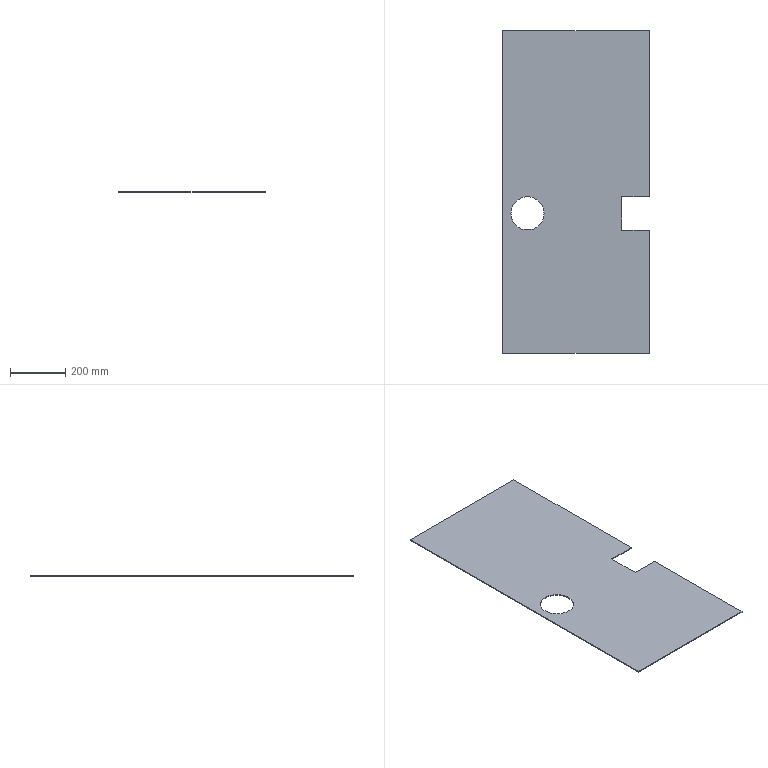Part | SolidWorks | features Cut 1, Extrusion 1 | 1 solid | 12 faces | box 530 x 1165 x 3 mm | volume 1782421 mm3 | plane 10 | cylinder 2 | commonest cylinder face diameters 120 x2
STEP:
#1=CARTESIAN_POINT('',(150.,505.,3.));
#2=VERTEX_POINT('',#1);
#3=CARTESIAN_POINT('',(30.,505.,3.));
#4=VERTEX_POINT('',#3);
#5=CARTESIAN_POINT('',(90.,505.,3.));
#6=DIRECTION('',(0.,0.,-1.));
#7=DIRECTION('',(-1.,0.,0.));
#8=AXIS2_PLACEMENT_3D('',#5,#6,#7);
#9=CIRCLE('',#8,60.);
#10=EDGE_CURVE('',#2,#4,#9,.T.);
#11=ORIENTED_EDGE('',*,*,#10,.F.);
#12=CARTESIAN_POINT('',(150.,505.,0.));
#13=VERTEX_POINT('',#12);
#14=CARTESIAN_POINT('',(150.,505.,10.));
#15=DIRECTION('',(0.,0.,-1.));
#16=VECTOR('',#15,1000.);
#17=LINE('',#14,#16);
#18=EDGE_CURVE('',#2,#13,#17,.T.);
#19=ORIENTED_EDGE('',*,*,#18,.T.);
#20=CARTESIAN_POINT('',(30.,505.,0.));
#21=VERTEX_POINT('',#20);
#22=CARTESIAN_POINT('',(90.,505.,0.));
#23=DIRECTION('',(0.,0.,-1.));
#24=DIRECTION('',(-1.,0.,0.));
#25=AXIS2_PLACEMENT_3D('',#22,#23,#24);
#26=CIRCLE('',#25,60.);
#27=EDGE_CURVE('',#13,#21,#26,.T.);
#28=ORIENTED_EDGE('',*,*,#27,.T.);
#29=CARTESIAN_POINT('',(30.,505.,10.));
#30=DIRECTION('',(0.,0.,-1.));
#31=VECTOR('',#30,1000.);
#32=LINE('',#29,#31);
#33=EDGE_CURVE('',#4,#21,#32,.T.);
#34=ORIENTED_EDGE('',*,*,#33,.F.);
#35=EDGE_LOOP('',(#11,#19,#28,#34));
#36=FACE_OUTER_BOUND('',#35,.T.);
#37=CARTESIAN_POINT('',(90.,505.,10.));
#38=DIRECTION('',(0.,0.,-1.));
#39=DIRECTION('',(-1.,0.,0.));
#40=AXIS2_PLACEMENT_3D('',#37,#38,#39);
#41=CYLINDRICAL_SURFACE('',#40,60.);
#42=ADVANCED_FACE('',(#36),#41,.F.);
#43=CARTESIAN_POINT('',(530.,565.,3.));
#44=VERTEX_POINT('',#43);
#45=CARTESIAN_POINT('',(530.,1165.,3.));
#46=VERTEX_POINT('',#45);
#47=CARTESIAN_POINT('',(530.,0.,3.));
#48=DIRECTION('',(0.,1.,0.));
#49=VECTOR('',#48,1000.);
#50=LINE('',#47,#49);
#51=EDGE_CURVE('',#44,#46,#50,.T.);
#52=ORIENTED_EDGE('',*,*,#51,.F.);
#53=CARTESIAN_POINT('',(530.,565.,0.));
#54=VERTEX_POINT('',#53);
#55=CARTESIAN_POINT('',(530.,565.,3.));
#56=DIRECTION('',(0.,0.,-1.));
#57=VECTOR('',#56,1000.);
#58=LINE('',#55,#57);
#59=EDGE_CURVE('',#44,#54,#58,.T.);
#60=ORIENTED_EDGE('',*,*,#59,.T.);
#61=CARTESIAN_POINT('',(530.,1165.,0.));
#62=VERTEX_POINT('',#61);
#63=CARTESIAN_POINT('',(530.,0.,0.));
#64=DIRECTION('',(0.,1.,0.));
#65=VECTOR('',#64,1000.);
#66=LINE('',#63,#65);
#67=EDGE_CURVE('',#54,#62,#66,.T.);
#68=ORIENTED_EDGE('',*,*,#67,.T.);
#69=CARTESIAN_POINT('',(530.,1165.,3.));
#70=DIRECTION('',(0.,0.,-1.));
#71=VECTOR('',#70,1000.);
#72=LINE('',#69,#71);
#73=EDGE_CURVE('',#46,#62,#72,.T.);
#74=ORIENTED_EDGE('',*,*,#73,.F.);
#75=EDGE_LOOP('',(#52,#60,#68,#74));
#76=FACE_OUTER_BOUND('',#75,.T.);
#77=CARTESIAN_POINT('',(530.,0.,3.));
#78=DIRECTION('',(-1.,0.,0.));
#79=DIRECTION('',(0.,0.,1.));
#80=AXIS2_PLACEMENT_3D('',#77,#78,#79);
#81=PLANE('',#80);
#82=ADVANCED_FACE('',(#76),#81,.F.);
#83=CARTESIAN_POINT('',(0.,1165.,0.));
#84=VERTEX_POINT('',#83);
#85=CARTESIAN_POINT('',(0.,0.,0.));
#86=VERTEX_POINT('',#85);
#87=CARTESIAN_POINT('',(0.,0.,0.));
#88=DIRECTION('',(0.,-1.,0.));
#89=VECTOR('',#88,1000.);
#90=LINE('',#87,#89);
#91=EDGE_CURVE('',#84,#86,#90,.T.);
#92=ORIENTED_EDGE('',*,*,#91,.T.);
#93=CARTESIAN_POINT('',(0.,0.,3.));
#94=VERTEX_POINT('',#93);
#95=CARTESIAN_POINT('',(0.,0.,3.));
#96=DIRECTION('',(0.,0.,-1.));
#97=VECTOR('',#96,1000.);
#98=LINE('',#95,#97);
#99=EDGE_CURVE('',#94,#86,#98,.T.);
#100=ORIENTED_EDGE('',*,*,#99,.F.);
#101=CARTESIAN_POINT('',(0.,1165.,3.));
#102=VERTEX_POINT('',#101);
#103=CARTESIAN_POINT('',(0.,0.,3.));
#104=DIRECTION('',(0.,-1.,0.));
#105=VECTOR('',#104,1000.);
#106=LINE('',#103,#105);
#107=EDGE_CURVE('',#102,#94,#106,.T.);
#108=ORIENTED_EDGE('',*,*,#107,.F.);
#109=CARTESIAN_POINT('',(0.,1165.,3.));
#110=DIRECTION('',(0.,0.,-1.));
#111=VECTOR('',#110,1000.);
#112=LINE('',#109,#111);
#113=EDGE_CURVE('',#102,#84,#112,.T.);
#114=ORIENTED_EDGE('',*,*,#113,.T.);
#115=EDGE_LOOP('',(#92,#100,#108,#114));
#116=FACE_OUTER_BOUND('',#115,.T.);
#117=CARTESIAN_POINT('',(0.,0.,3.));
#118=DIRECTION('',(1.,0.,0.));
#119=DIRECTION('',(0.,0.,-1.));
#120=AXIS2_PLACEMENT_3D('',#117,#118,#119);
#121=PLANE('',#120);
#122=ADVANCED_FACE('',(#116),#121,.F.);
#123=CARTESIAN_POINT('',(530.,0.,0.));
#124=VERTEX_POINT('',#123);
#125=CARTESIAN_POINT('',(0.,0.,0.));
#126=DIRECTION('',(1.,0.,0.));
#127=VECTOR('',#126,1000.);
#128=LINE('',#125,#127);
#129=EDGE_CURVE('',#86,#124,#128,.T.);
#130=ORIENTED_EDGE('',*,*,#129,.T.);
#131=CARTESIAN_POINT('',(530.,0.,3.));
#132=VERTEX_POINT('',#131);
#133=CARTESIAN_POINT('',(530.,0.,3.));
#134=DIRECTION('',(0.,0.,-1.));
#135=VECTOR('',#134,1000.);
#136=LINE('',#133,#135);
#137=EDGE_CURVE('',#132,#124,#136,.T.);
#138=ORIENTED_EDGE('',*,*,#137,.F.);
#139=CARTESIAN_POINT('',(0.,0.,3.));
#140=DIRECTION('',(1.,0.,0.));
#141=VECTOR('',#140,1000.);
#142=LINE('',#139,#141);
#143=EDGE_CURVE('',#94,#132,#142,.T.);
#144=ORIENTED_EDGE('',*,*,#143,.F.);
#145=ORIENTED_EDGE('',*,*,#99,.T.);
#146=EDGE_LOOP('',(#130,#138,#144,#145));
#147=FACE_OUTER_BOUND('',#146,.T.);
#148=CARTESIAN_POINT('',(0.,0.,3.));
#149=DIRECTION('',(0.,1.,0.));
#150=DIRECTION('',(0.,0.,1.));
#151=AXIS2_PLACEMENT_3D('',#148,#149,#150);
#152=PLANE('',#151);
#153=ADVANCED_FACE('',(#147),#152,.F.);
#154=CARTESIAN_POINT('',(530.,445.,0.));
#155=VERTEX_POINT('',#154);
#156=CARTESIAN_POINT('',(530.,0.,0.));
#157=DIRECTION('',(0.,1.,0.));
#158=VECTOR('',#157,1000.);
#159=LINE('',#156,#158);
#160=EDGE_CURVE('',#124,#155,#159,.T.);
#161=ORIENTED_EDGE('',*,*,#160,.T.);
#162=CARTESIAN_POINT('',(530.,445.,3.));
#163=VERTEX_POINT('',#162);
#164=CARTESIAN_POINT('',(530.,445.,3.));
#165=DIRECTION('',(0.,0.,1.));
#166=VECTOR('',#165,1000.);
#167=LINE('',#164,#166);
#168=EDGE_CURVE('',#155,#163,#167,.T.);
#169=ORIENTED_EDGE('',*,*,#168,.T.);
#170=CARTESIAN_POINT('',(530.,0.,3.));
#171=DIRECTION('',(0.,1.,0.));
#172=VECTOR('',#171,1000.);
#173=LINE('',#170,#172);
#174=EDGE_CURVE('',#132,#163,#173,.T.);
#175=ORIENTED_EDGE('',*,*,#174,.F.);
#176=ORIENTED_EDGE('',*,*,#137,.T.);
#177=EDGE_LOOP('',(#161,#169,#175,#176));
#178=FACE_OUTER_BOUND('',#177,.T.);
#179=CARTESIAN_POINT('',(530.,0.,3.));
#180=DIRECTION('',(-1.,0.,0.));
#181=DIRECTION('',(0.,0.,1.));
#182=AXIS2_PLACEMENT_3D('',#179,#180,#181);
#183=PLANE('',#182);
#184=ADVANCED_FACE('',(#178),#183,.F.);
#185=CARTESIAN_POINT('',(0.,1165.,0.));
#186=DIRECTION('',(-1.,0.,0.));
#187=VECTOR('',#186,1000.);
#188=LINE('',#185,#187);
#189=EDGE_CURVE('',#62,#84,#188,.T.);
#190=ORIENTED_EDGE('',*,*,#189,.T.);
#191=ORIENTED_EDGE('',*,*,#113,.F.);
#192=CARTESIAN_POINT('',(0.,1165.,3.));
#193=DIRECTION('',(-1.,0.,0.));
#194=VECTOR('',#193,1000.);
#195=LINE('',#192,#194);
#196=EDGE_CURVE('',#46,#102,#195,.T.);
#197=ORIENTED_EDGE('',*,*,#196,.F.);
#198=ORIENTED_EDGE('',*,*,#73,.T.);
#199=EDGE_LOOP('',(#190,#191,#197,#198));
#200=FACE_OUTER_BOUND('',#199,.T.);
#201=CARTESIAN_POINT('',(0.,1165.,3.));
#202=DIRECTION('',(0.,-1.,0.));
#203=DIRECTION('',(0.,0.,-1.));
#204=AXIS2_PLACEMENT_3D('',#201,#202,#203);
#205=PLANE('',#204);
#206=ADVANCED_FACE('',(#200),#205,.F.);
#207=CARTESIAN_POINT('',(90.,505.,3.));
#208=DIRECTION('',(0.,0.,-1.));
#209=DIRECTION('',(-1.,0.,0.));
#210=AXIS2_PLACEMENT_3D('',#207,#208,#209);
#211=CIRCLE('',#210,60.);
#212=EDGE_CURVE('',#4,#2,#211,.T.);
#213=ORIENTED_EDGE('',*,*,#212,.T.);
#214=ORIENTED_EDGE('',*,*,#10,.T.);
#215=EDGE_LOOP('',(#213,#214));
#216=FACE_BOUND('',#215,.T.);
#217=CARTESIAN_POINT('',(430.,445.,3.));
#218=VERTEX_POINT('',#217);
#219=CARTESIAN_POINT('',(430.,565.,3.));
#220=VERTEX_POINT('',#219);
#221=CARTESIAN_POINT('',(430.,0.,3.));
#222=DIRECTION('',(0.,1.,0.));
#223=VECTOR('',#222,1000.);
#224=LINE('',#221,#223);
#225=EDGE_CURVE('',#218,#220,#224,.T.);
#226=ORIENTED_EDGE('',*,*,#225,.T.);
#227=CARTESIAN_POINT('',(0.,565.,3.));
#228=DIRECTION('',(1.,0.,0.));
#229=VECTOR('',#228,1000.);
#230=LINE('',#227,#229);
#231=EDGE_CURVE('',#220,#44,#230,.T.);
#232=ORIENTED_EDGE('',*,*,#231,.T.);
#233=ORIENTED_EDGE('',*,*,#51,.T.);
#234=ORIENTED_EDGE('',*,*,#196,.T.);
#235=ORIENTED_EDGE('',*,*,#107,.T.);
#236=ORIENTED_EDGE('',*,*,#143,.T.);
#237=ORIENTED_EDGE('',*,*,#174,.T.);
#238=CARTESIAN_POINT('',(0.,445.,3.));
#239=DIRECTION('',(-1.,0.,0.));
#240=VECTOR('',#239,1000.);
#241=LINE('',#238,#240);
#242=EDGE_CURVE('',#163,#218,#241,.T.);
#243=ORIENTED_EDGE('',*,*,#242,.T.);
#244=EDGE_LOOP('',(#226,#232,#233,#234,#235,#236,#237,#243));
#245=FACE_OUTER_BOUND('',#244,.T.);
#246=CARTESIAN_POINT('',(0.,0.,3.));
#247=DIRECTION('',(0.,0.,-1.));
#248=DIRECTION('',(-1.,0.,0.));
#249=AXIS2_PLACEMENT_3D('',#246,#247,#248);
#250=PLANE('',#249);
#251=ADVANCED_FACE('',(#216,#245),#250,.F.);
#252=CARTESIAN_POINT('',(90.,505.,0.));
#253=DIRECTION('',(0.,0.,-1.));
#254=DIRECTION('',(-1.,0.,0.));
#255=AXIS2_PLACEMENT_3D('',#252,#253,#254);
#256=CIRCLE('',#255,60.);
#257=EDGE_CURVE('',#21,#13,#256,.T.);
#258=ORIENTED_EDGE('',*,*,#257,.F.);
#259=ORIENTED_EDGE('',*,*,#27,.F.);
#260=EDGE_LOOP('',(#258,#259));
#261=FACE_BOUND('',#260,.T.);
#262=CARTESIAN_POINT('',(430.,565.,0.));
#263=VERTEX_POINT('',#262);
#264=CARTESIAN_POINT('',(430.,565.,0.));
#265=DIRECTION('',(1.,0.,0.));
#266=VECTOR('',#265,1000.);
#267=LINE('',#264,#266);
#268=EDGE_CURVE('',#263,#54,#267,.T.);
#269=ORIENTED_EDGE('',*,*,#268,.F.);
#270=CARTESIAN_POINT('',(430.,445.,0.));
#271=VERTEX_POINT('',#270);
#272=CARTESIAN_POINT('',(430.,445.,0.));
#273=DIRECTION('',(0.,1.,0.));
#274=VECTOR('',#273,1000.);
#275=LINE('',#272,#274);
#276=EDGE_CURVE('',#271,#263,#275,.T.);
#277=ORIENTED_EDGE('',*,*,#276,.F.);
#278=CARTESIAN_POINT('',(0.,445.,0.));
#279=DIRECTION('',(-1.,0.,0.));
#280=VECTOR('',#279,1000.);
#281=LINE('',#278,#280);
#282=EDGE_CURVE('',#155,#271,#281,.T.);
#283=ORIENTED_EDGE('',*,*,#282,.F.);
#284=ORIENTED_EDGE('',*,*,#160,.F.);
#285=ORIENTED_EDGE('',*,*,#129,.F.);
#286=ORIENTED_EDGE('',*,*,#91,.F.);
#287=ORIENTED_EDGE('',*,*,#189,.F.);
#288=ORIENTED_EDGE('',*,*,#67,.F.);
#289=EDGE_LOOP('',(#269,#277,#283,#284,#285,#286,#287,#288));
#290=FACE_OUTER_BOUND('',#289,.T.);
#291=CARTESIAN_POINT('',(0.,0.,0.));
#292=DIRECTION('',(0.,0.,-1.));
#293=DIRECTION('',(-1.,0.,0.));
#294=AXIS2_PLACEMENT_3D('',#291,#292,#293);
#295=PLANE('',#294);
#296=ADVANCED_FACE('',(#261,#290),#295,.T.);
#297=ORIENTED_EDGE('',*,*,#231,.F.);
#298=CARTESIAN_POINT('',(430.,565.,10.));
#299=DIRECTION('',(0.,0.,-1.));
#300=VECTOR('',#299,1000.);
#301=LINE('',#298,#300);
#302=EDGE_CURVE('',#220,#263,#301,.T.);
#303=ORIENTED_EDGE('',*,*,#302,.T.);
#304=ORIENTED_EDGE('',*,*,#268,.T.);
#305=ORIENTED_EDGE('',*,*,#59,.F.);
#306=EDGE_LOOP('',(#297,#303,#304,#305));
#307=FACE_OUTER_BOUND('',#306,.T.);
#308=CARTESIAN_POINT('',(430.,565.,10.));
#309=DIRECTION('',(0.,1.,0.));
#310=DIRECTION('',(0.,0.,1.));
#311=AXIS2_PLACEMENT_3D('',#308,#309,#310);
#312=PLANE('',#311);
#313=ADVANCED_FACE('',(#307),#312,.F.);
#314=CARTESIAN_POINT('',(430.,445.,10.));
#315=DIRECTION('',(0.,0.,-1.));
#316=VECTOR('',#315,1000.);
#317=LINE('',#314,#316);
#318=EDGE_CURVE('',#218,#271,#317,.T.);
#319=ORIENTED_EDGE('',*,*,#318,.T.);
#320=ORIENTED_EDGE('',*,*,#276,.T.);
#321=ORIENTED_EDGE('',*,*,#302,.F.);
#322=ORIENTED_EDGE('',*,*,#225,.F.);
#323=EDGE_LOOP('',(#319,#320,#321,#322));
#324=FACE_OUTER_BOUND('',#323,.T.);
#325=CARTESIAN_POINT('',(430.,445.,10.));
#326=DIRECTION('',(-1.,0.,0.));
#327=DIRECTION('',(0.,0.,1.));
#328=AXIS2_PLACEMENT_3D('',#325,#326,#327);
#329=PLANE('',#328);
#330=ADVANCED_FACE('',(#324),#329,.F.);
#331=ORIENTED_EDGE('',*,*,#282,.T.);
#332=ORIENTED_EDGE('',*,*,#318,.F.);
#333=ORIENTED_EDGE('',*,*,#242,.F.);
#334=ORIENTED_EDGE('',*,*,#168,.F.);
#335=EDGE_LOOP('',(#331,#332,#333,#334));
#336=FACE_OUTER_BOUND('',#335,.T.);
#337=CARTESIAN_POINT('',(430.,445.,10.));
#338=DIRECTION('',(0.,-1.,0.));
#339=DIRECTION('',(0.,0.,-1.));
#340=AXIS2_PLACEMENT_3D('',#337,#338,#339);
#341=PLANE('',#340);
#342=ADVANCED_FACE('',(#336),#341,.F.);
#343=ORIENTED_EDGE('',*,*,#18,.F.);
#344=ORIENTED_EDGE('',*,*,#212,.F.);
#345=ORIENTED_EDGE('',*,*,#33,.T.);
#346=ORIENTED_EDGE('',*,*,#257,.T.);
#347=EDGE_LOOP('',(#343,#344,#345,#346));
#348=FACE_OUTER_BOUND('',#347,.T.);
#349=CARTESIAN_POINT('',(90.,505.,10.));
#350=DIRECTION('',(0.,0.,-1.));
#351=DIRECTION('',(-1.,0.,0.));
#352=AXIS2_PLACEMENT_3D('',#349,#350,#351);
#353=CYLINDRICAL_SURFACE('',#352,60.);
#354=ADVANCED_FACE('',(#348),#353,.F.);
#355=CLOSED_SHELL('',(#42,#82,#122,#153,#184,#206,#251,#296,#313,#330,#342,#354));
#356=MANIFOLD_SOLID_BREP('',#355);
#357=CARTESIAN_POINT('',(0.,0.,0.));
#358=DIRECTION('',(0.,0.,1.));
#359=DIRECTION('',(1.,0.,0.));
#360=AXIS2_PLACEMENT_3D('',#357,#358,#359);
#361=(LENGTH_UNIT()NAMED_UNIT(*)SI_UNIT(.MILLI.,.METRE.));
#362=UNCERTAINTY_MEASURE_WITH_UNIT(LENGTH_MEASURE(0.00001),#361,'','');
#363=(NAMED_UNIT(*)PLANE_ANGLE_UNIT()SI_UNIT($,.RADIAN.));
#364=(NAMED_UNIT(*)SI_UNIT($,.STERADIAN.)SOLID_ANGLE_UNIT());
#365=(GEOMETRIC_REPRESENTATION_CONTEXT(3)GLOBAL_UNCERTAINTY_ASSIGNED_CONTEXT((#362))GLOBAL_UNIT_ASSIGNED_CONTEXT((#361,#363,#364))REPRESENTATION_CONTEXT('',''));
#366=ADVANCED_BREP_SHAPE_REPRESENTATION('',(#356,#360),#365);